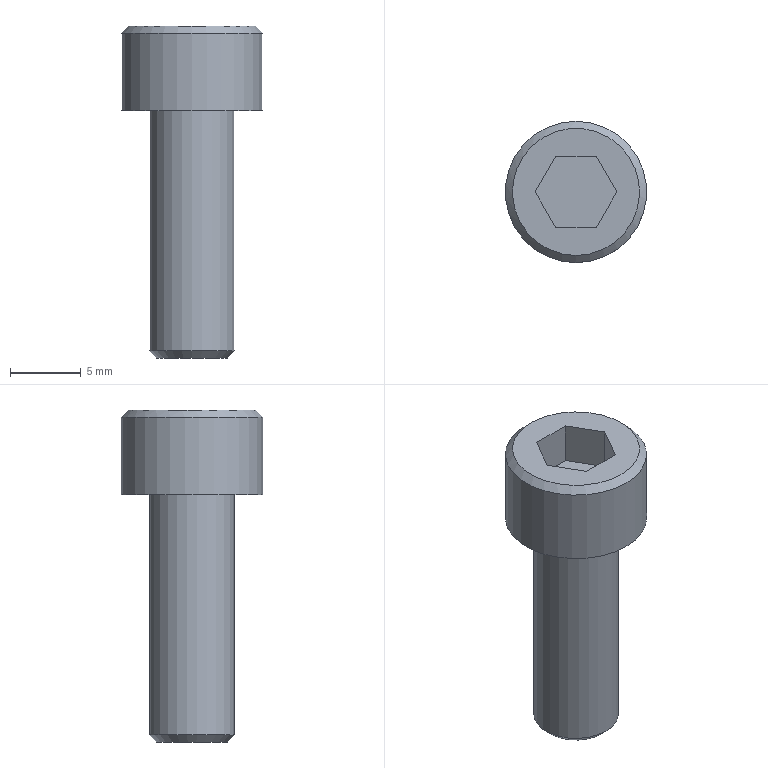Part | STEP file | solid 126 | 1 solid | 14 faces | box 10 x 10 x 23.5 mm | volume 895.066 mm3 | plane 10 | cone 2 | cylinder 2 | commonest cylinder face diameters 6 x1 10 x1